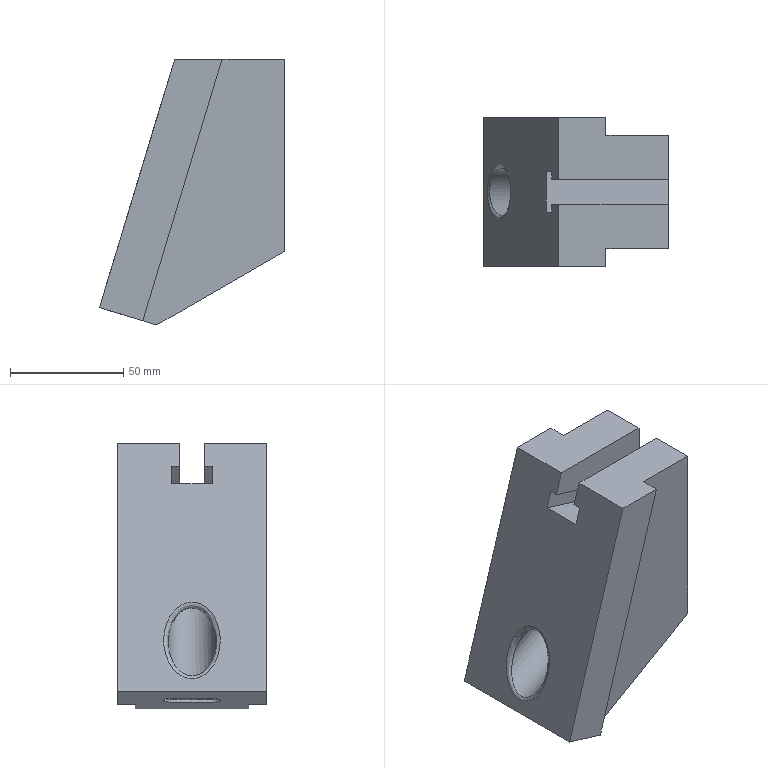Part | STEP file | solid 248 | 1 solid | 99 faces | box 81.775 x 66 x 117.55 mm | volume 328210 mm3 | plane 55 | other 39 | cylinder 3 | spline 2 | commonest cylinder face diameters 6 x2 21 x1